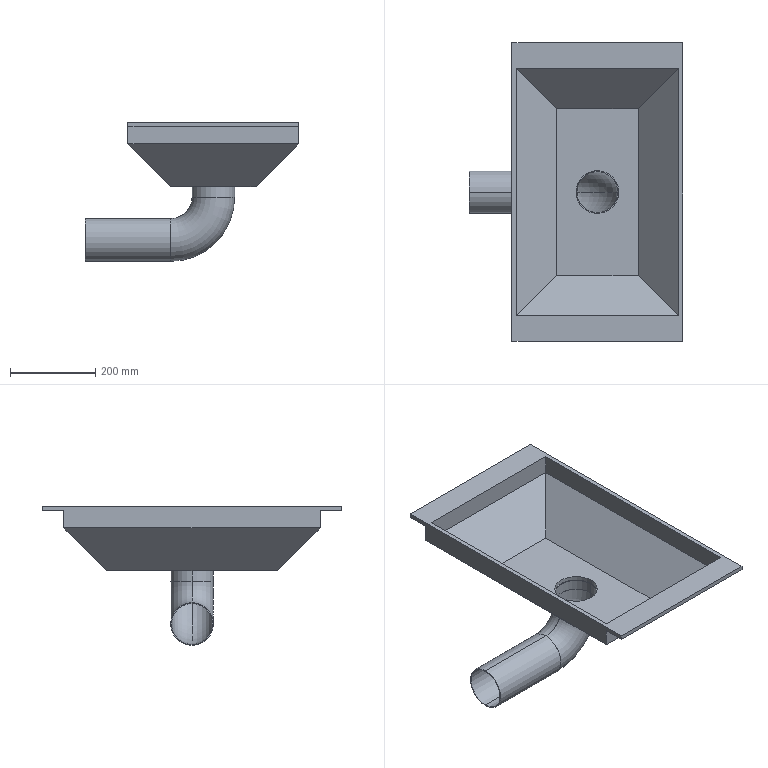Part | SolidWorks | features ICE 4, Shell 2, Chamfer 1, Extrusion 1, Sweep 1 | 2 solids | 39 faces | box 500 x 700 x 325 mm | volume 4429815 mm3 | plane 25 | cylinder 10 | torus 4 | commonest cylinder face diameters 100 x6 96 x4
STEP:
#1=CARTESIAN_POINT('',(48.,0.,-25.));
#2=VERTEX_POINT('',#1);
#3=CARTESIAN_POINT('',(-48.,0.,-25.));
#4=VERTEX_POINT('',#3);
#5=CARTESIAN_POINT('',(0.,0.,-25.));
#6=DIRECTION('',(0.,0.,-1.));
#7=DIRECTION('',(1.,0.,0.));
#8=AXIS2_PLACEMENT_3D('',#5,#6,#7);
#9=CIRCLE('',#8,48.);
#10=EDGE_CURVE('',#2,#4,#9,.T.);
#11=ORIENTED_EDGE('',*,*,#10,.F.);
#12=CARTESIAN_POINT('',(-100.,0.,-173.));
#13=VERTEX_POINT('',#12);
#14=CARTESIAN_POINT('',(-100.,0.,-25.));
#15=DIRECTION('',(0.,1.,0.));
#16=DIRECTION('',(0.,0.,1.));
#17=AXIS2_PLACEMENT_3D('',#14,#15,#16);
#18=CIRCLE('',#17,148.);
#19=EDGE_CURVE('',#2,#13,#18,.T.);
#20=ORIENTED_EDGE('',*,*,#19,.T.);
#21=CARTESIAN_POINT('',(-100.,0.,-77.));
#22=VERTEX_POINT('',#21);
#23=CARTESIAN_POINT('',(-100.,0.,-125.));
#24=DIRECTION('',(-1.,0.,0.));
#25=DIRECTION('',(0.,0.,1.));
#26=AXIS2_PLACEMENT_3D('',#23,#24,#25);
#27=CIRCLE('',#26,48.);
#28=EDGE_CURVE('',#13,#22,#27,.T.);
#29=ORIENTED_EDGE('',*,*,#28,.T.);
#30=CARTESIAN_POINT('',(-100.,0.,-25.));
#31=DIRECTION('',(0.,1.,0.));
#32=DIRECTION('',(0.,0.,1.));
#33=AXIS2_PLACEMENT_3D('',#30,#31,#32);
#34=CIRCLE('',#33,52.);
#35=EDGE_CURVE('',#4,#22,#34,.T.);
#36=ORIENTED_EDGE('',*,*,#35,.F.);
#37=EDGE_LOOP('',(#11,#20,#29,#36));
#38=FACE_OUTER_BOUND('',#37,.T.);
#39=CARTESIAN_POINT('',(-100.,0.,-25.));
#40=DIRECTION('',(0.,1.,0.));
#41=DIRECTION('',(0.,0.,1.));
#42=AXIS2_PLACEMENT_3D('',#39,#40,#41);
#43=TOROIDAL_SURFACE('',#42,100.,48.);
#44=ADVANCED_FACE('',(#38),#43,.F.);
#45=CARTESIAN_POINT('',(-50.,0.,-25.));
#46=VERTEX_POINT('',#45);
#47=CARTESIAN_POINT('',(50.,0.,-25.));
#48=VERTEX_POINT('',#47);
#49=CARTESIAN_POINT('',(0.,0.,-25.));
#50=DIRECTION('',(0.,0.,-1.));
#51=DIRECTION('',(-1.,0.,0.));
#52=AXIS2_PLACEMENT_3D('',#49,#50,#51);
#53=CIRCLE('',#52,50.);
#54=EDGE_CURVE('',#46,#48,#53,.T.);
#55=ORIENTED_EDGE('',*,*,#54,.T.);
#56=CARTESIAN_POINT('',(-100.,0.,-175.));
#57=VERTEX_POINT('',#56);
#58=CARTESIAN_POINT('',(-100.,0.,-25.));
#59=DIRECTION('',(0.,1.,0.));
#60=DIRECTION('',(0.,0.,1.));
#61=AXIS2_PLACEMENT_3D('',#58,#59,#60);
#62=CIRCLE('',#61,150.);
#63=EDGE_CURVE('',#48,#57,#62,.T.);
#64=ORIENTED_EDGE('',*,*,#63,.T.);
#65=CARTESIAN_POINT('',(-100.,0.,-75.));
#66=VERTEX_POINT('',#65);
#67=CARTESIAN_POINT('',(-100.,0.,-125.));
#68=DIRECTION('',(-1.,0.,0.));
#69=DIRECTION('',(0.,0.,1.));
#70=AXIS2_PLACEMENT_3D('',#67,#68,#69);
#71=CIRCLE('',#70,50.);
#72=EDGE_CURVE('',#66,#57,#71,.T.);
#73=ORIENTED_EDGE('',*,*,#72,.F.);
#74=CARTESIAN_POINT('',(-100.,0.,-25.));
#75=DIRECTION('',(0.,1.,0.));
#76=DIRECTION('',(0.,0.,1.));
#77=AXIS2_PLACEMENT_3D('',#74,#75,#76);
#78=CIRCLE('',#77,50.);
#79=EDGE_CURVE('',#46,#66,#78,.T.);
#80=ORIENTED_EDGE('',*,*,#79,.F.);
#81=EDGE_LOOP('',(#55,#64,#73,#80));
#82=FACE_OUTER_BOUND('',#81,.T.);
#83=CARTESIAN_POINT('',(-100.,0.,-25.));
#84=DIRECTION('',(0.,1.,0.));
#85=DIRECTION('',(0.,0.,1.));
#86=AXIS2_PLACEMENT_3D('',#83,#84,#85);
#87=TOROIDAL_SURFACE('',#86,100.,50.);
#88=ADVANCED_FACE('',(#82),#87,.T.);
#89=ORIENTED_EDGE('',*,*,#28,.F.);
#90=CARTESIAN_POINT('',(-300.,0.,-173.));
#91=VERTEX_POINT('',#90);
#92=CARTESIAN_POINT('',(-100.,0.,-173.));
#93=DIRECTION('',(-1.,0.,0.));
#94=VECTOR('',#93,1000.);
#95=LINE('',#92,#94);
#96=EDGE_CURVE('',#13,#91,#95,.T.);
#97=ORIENTED_EDGE('',*,*,#96,.T.);
#98=CARTESIAN_POINT('',(-300.,0.,-77.));
#99=VERTEX_POINT('',#98);
#100=CARTESIAN_POINT('',(-300.,0.,-125.));
#101=DIRECTION('',(-1.,0.,0.));
#102=DIRECTION('',(0.,0.,1.));
#103=AXIS2_PLACEMENT_3D('',#100,#101,#102);
#104=CIRCLE('',#103,48.);
#105=EDGE_CURVE('',#91,#99,#104,.T.);
#106=ORIENTED_EDGE('',*,*,#105,.T.);
#107=CARTESIAN_POINT('',(-100.,0.,-77.));
#108=DIRECTION('',(-1.,0.,0.));
#109=VECTOR('',#108,1000.);
#110=LINE('',#107,#109);
#111=EDGE_CURVE('',#22,#99,#110,.T.);
#112=ORIENTED_EDGE('',*,*,#111,.F.);
#113=EDGE_LOOP('',(#89,#97,#106,#112));
#114=FACE_OUTER_BOUND('',#113,.T.);
#115=CARTESIAN_POINT('',(-100.,0.,-125.));
#116=DIRECTION('',(-1.,0.,0.));
#117=DIRECTION('',(0.,0.,1.));
#118=AXIS2_PLACEMENT_3D('',#115,#116,#117);
#119=CYLINDRICAL_SURFACE('',#118,48.);
#120=ADVANCED_FACE('',(#114),#119,.F.);
#121=CARTESIAN_POINT('',(48.,0.,0.));
#122=VERTEX_POINT('',#121);
#123=CARTESIAN_POINT('',(-48.,0.,0.));
#124=VERTEX_POINT('',#123);
#125=CARTESIAN_POINT('',(0.,0.,0.));
#126=DIRECTION('',(0.,0.,-1.));
#127=DIRECTION('',(-1.,0.,0.));
#128=AXIS2_PLACEMENT_3D('',#125,#126,#127);
#129=CIRCLE('',#128,48.);
#130=EDGE_CURVE('',#122,#124,#129,.T.);
#131=ORIENTED_EDGE('',*,*,#130,.F.);
#132=CARTESIAN_POINT('',(48.,0.,0.));
#133=DIRECTION('',(0.,0.,-1.));
#134=VECTOR('',#133,1000.);
#135=LINE('',#132,#134);
#136=EDGE_CURVE('',#122,#2,#135,.T.);
#137=ORIENTED_EDGE('',*,*,#136,.T.);
#138=ORIENTED_EDGE('',*,*,#10,.T.);
#139=CARTESIAN_POINT('',(-48.,0.,0.));
#140=DIRECTION('',(0.,0.,-1.));
#141=VECTOR('',#140,1000.);
#142=LINE('',#139,#141);
#143=EDGE_CURVE('',#124,#4,#142,.T.);
#144=ORIENTED_EDGE('',*,*,#143,.F.);
#145=EDGE_LOOP('',(#131,#137,#138,#144));
#146=FACE_OUTER_BOUND('',#145,.T.);
#147=CARTESIAN_POINT('',(0.,0.,0.));
#148=DIRECTION('',(0.,0.,-1.));
#149=DIRECTION('',(-1.,0.,0.));
#150=AXIS2_PLACEMENT_3D('',#147,#148,#149);
#151=CYLINDRICAL_SURFACE('',#150,48.);
#152=ADVANCED_FACE('',(#146),#151,.F.);
#153=ORIENTED_EDGE('',*,*,#72,.T.);
#154=CARTESIAN_POINT('',(-300.,0.,-175.));
#155=VERTEX_POINT('',#154);
#156=CARTESIAN_POINT('',(-100.,0.,-175.));
#157=DIRECTION('',(-1.,0.,0.));
#158=VECTOR('',#157,1000.);
#159=LINE('',#156,#158);
#160=EDGE_CURVE('',#57,#155,#159,.T.);
#161=ORIENTED_EDGE('',*,*,#160,.T.);
#162=CARTESIAN_POINT('',(-300.,0.,-75.));
#163=VERTEX_POINT('',#162);
#164=CARTESIAN_POINT('',(-300.,0.,-125.));
#165=DIRECTION('',(-1.,0.,0.));
#166=DIRECTION('',(0.,0.,1.));
#167=AXIS2_PLACEMENT_3D('',#164,#165,#166);
#168=CIRCLE('',#167,50.);
#169=EDGE_CURVE('',#163,#155,#168,.T.);
#170=ORIENTED_EDGE('',*,*,#169,.F.);
#171=CARTESIAN_POINT('',(-100.,0.,-75.));
#172=DIRECTION('',(-1.,0.,0.));
#173=VECTOR('',#172,1000.);
#174=LINE('',#171,#173);
#175=EDGE_CURVE('',#66,#163,#174,.T.);
#176=ORIENTED_EDGE('',*,*,#175,.F.);
#177=EDGE_LOOP('',(#153,#161,#170,#176));
#178=FACE_OUTER_BOUND('',#177,.T.);
#179=CARTESIAN_POINT('',(-100.,0.,-125.));
#180=DIRECTION('',(-1.,0.,0.));
#181=DIRECTION('',(0.,0.,1.));
#182=AXIS2_PLACEMENT_3D('',#179,#180,#181);
#183=CYLINDRICAL_SURFACE('',#182,50.);
#184=ADVANCED_FACE('',(#178),#183,.T.);
#185=CARTESIAN_POINT('',(-50.,0.,0.));
#186=VERTEX_POINT('',#185);
#187=CARTESIAN_POINT('',(50.,0.,0.));
#188=VERTEX_POINT('',#187);
#189=CARTESIAN_POINT('',(0.,0.,0.));
#190=DIRECTION('',(0.,0.,-1.));
#191=DIRECTION('',(-1.,0.,0.));
#192=AXIS2_PLACEMENT_3D('',#189,#190,#191);
#193=CIRCLE('',#192,50.);
#194=EDGE_CURVE('',#186,#188,#193,.T.);
#195=ORIENTED_EDGE('',*,*,#194,.T.);
#196=CARTESIAN_POINT('',(50.,0.,0.));
#197=DIRECTION('',(0.,0.,-1.));
#198=VECTOR('',#197,1000.);
#199=LINE('',#196,#198);
#200=EDGE_CURVE('',#188,#48,#199,.T.);
#201=ORIENTED_EDGE('',*,*,#200,.T.);
#202=ORIENTED_EDGE('',*,*,#54,.F.);
#203=CARTESIAN_POINT('',(-50.,0.,0.));
#204=DIRECTION('',(0.,0.,-1.));
#205=VECTOR('',#204,1000.);
#206=LINE('',#203,#205);
#207=EDGE_CURVE('',#186,#46,#206,.T.);
#208=ORIENTED_EDGE('',*,*,#207,.F.);
#209=EDGE_LOOP('',(#195,#201,#202,#208));
#210=FACE_OUTER_BOUND('',#209,.T.);
#211=CARTESIAN_POINT('',(0.,0.,0.));
#212=DIRECTION('',(0.,0.,-1.));
#213=DIRECTION('',(-1.,0.,0.));
#214=AXIS2_PLACEMENT_3D('',#211,#212,#213);
#215=CYLINDRICAL_SURFACE('',#214,50.);
#216=ADVANCED_FACE('',(#210),#215,.T.);
#217=ORIENTED_EDGE('',*,*,#160,.F.);
#218=CARTESIAN_POINT('',(-100.,0.,-125.));
#219=DIRECTION('',(-1.,0.,0.));
#220=DIRECTION('',(0.,0.,1.));
#221=AXIS2_PLACEMENT_3D('',#218,#219,#220);
#222=CIRCLE('',#221,50.);
#223=EDGE_CURVE('',#57,#66,#222,.T.);
#224=ORIENTED_EDGE('',*,*,#223,.T.);
#225=ORIENTED_EDGE('',*,*,#175,.T.);
#226=CARTESIAN_POINT('',(-300.,0.,-125.));
#227=DIRECTION('',(-1.,0.,0.));
#228=DIRECTION('',(0.,0.,1.));
#229=AXIS2_PLACEMENT_3D('',#226,#227,#228);
#230=CIRCLE('',#229,50.);
#231=EDGE_CURVE('',#155,#163,#230,.T.);
#232=ORIENTED_EDGE('',*,*,#231,.F.);
#233=EDGE_LOOP('',(#217,#224,#225,#232));
#234=FACE_OUTER_BOUND('',#233,.T.);
#235=CARTESIAN_POINT('',(-100.,0.,-125.));
#236=DIRECTION('',(-1.,0.,0.));
#237=DIRECTION('',(0.,0.,1.));
#238=AXIS2_PLACEMENT_3D('',#235,#236,#237);
#239=CYLINDRICAL_SURFACE('',#238,50.);
#240=ADVANCED_FACE('',(#234),#239,.T.);
#241=ORIENTED_EDGE('',*,*,#63,.F.);
#242=CARTESIAN_POINT('',(0.,0.,-25.));
#243=DIRECTION('',(0.,0.,-1.));
#244=DIRECTION('',(-1.,0.,0.));
#245=AXIS2_PLACEMENT_3D('',#242,#243,#244);
#246=CIRCLE('',#245,50.);
#247=EDGE_CURVE('',#48,#46,#246,.T.);
#248=ORIENTED_EDGE('',*,*,#247,.T.);
#249=ORIENTED_EDGE('',*,*,#79,.T.);
#250=ORIENTED_EDGE('',*,*,#223,.F.);
#251=EDGE_LOOP('',(#241,#248,#249,#250));
#252=FACE_OUTER_BOUND('',#251,.T.);
#253=CARTESIAN_POINT('',(-100.,0.,-25.));
#254=DIRECTION('',(0.,1.,0.));
#255=DIRECTION('',(0.,0.,1.));
#256=AXIS2_PLACEMENT_3D('',#253,#254,#255);
#257=TOROIDAL_SURFACE('',#256,100.,50.);
#258=ADVANCED_FACE('',(#252),#257,.T.);
#259=ORIENTED_EDGE('',*,*,#200,.F.);
#260=CARTESIAN_POINT('',(0.,0.,0.));
#261=DIRECTION('',(0.,0.,-1.));
#262=DIRECTION('',(-1.,0.,0.));
#263=AXIS2_PLACEMENT_3D('',#260,#261,#262);
#264=CIRCLE('',#263,50.);
#265=EDGE_CURVE('',#188,#186,#264,.T.);
#266=ORIENTED_EDGE('',*,*,#265,.T.);
#267=ORIENTED_EDGE('',*,*,#207,.T.);
#268=ORIENTED_EDGE('',*,*,#247,.F.);
#269=EDGE_LOOP('',(#259,#266,#267,#268));
#270=FACE_OUTER_BOUND('',#269,.T.);
#271=CARTESIAN_POINT('',(0.,0.,0.));
#272=DIRECTION('',(0.,0.,-1.));
#273=DIRECTION('',(-1.,0.,0.));
#274=AXIS2_PLACEMENT_3D('',#271,#272,#273);
#275=CYLINDRICAL_SURFACE('',#274,50.);
#276=ADVANCED_FACE('',(#270),#275,.T.);
#277=CARTESIAN_POINT('',(-300.,0.,-125.));
#278=DIRECTION('',(-1.,0.,0.));
#279=DIRECTION('',(0.,0.,1.));
#280=AXIS2_PLACEMENT_3D('',#277,#278,#279);
#281=CIRCLE('',#280,48.);
#282=EDGE_CURVE('',#99,#91,#281,.T.);
#283=ORIENTED_EDGE('',*,*,#282,.F.);
#284=ORIENTED_EDGE('',*,*,#105,.F.);
#285=EDGE_LOOP('',(#283,#284));
#286=FACE_BOUND('',#285,.T.);
#287=ORIENTED_EDGE('',*,*,#169,.T.);
#288=ORIENTED_EDGE('',*,*,#231,.T.);
#289=EDGE_LOOP('',(#287,#288));
#290=FACE_OUTER_BOUND('',#289,.T.);
#291=CARTESIAN_POINT('',(-300.,0.,-125.));
#292=DIRECTION('',(-1.,0.,0.));
#293=DIRECTION('',(0.,0.,1.));
#294=AXIS2_PLACEMENT_3D('',#291,#292,#293);
#295=PLANE('',#294);
#296=ADVANCED_FACE('',(#286,#290),#295,.T.);
#297=CARTESIAN_POINT('',(0.,0.,0.));
#298=DIRECTION('',(0.,0.,-1.));
#299=DIRECTION('',(-1.,0.,0.));
#300=AXIS2_PLACEMENT_3D('',#297,#298,#299);
#301=CIRCLE('',#300,48.);
#302=EDGE_CURVE('',#124,#122,#301,.T.);
#303=ORIENTED_EDGE('',*,*,#302,.T.);
#304=ORIENTED_EDGE('',*,*,#130,.T.);
#305=EDGE_LOOP('',(#303,#304));
#306=FACE_BOUND('',#305,.T.);
#307=ORIENTED_EDGE('',*,*,#194,.F.);
#308=ORIENTED_EDGE('',*,*,#265,.F.);
#309=EDGE_LOOP('',(#307,#308));
#310=FACE_OUTER_BOUND('',#309,.T.);
#311=CARTESIAN_POINT('',(0.,0.,0.));
#312=DIRECTION('',(0.,0.,-1.));
#313=DIRECTION('',(-1.,0.,0.));
#314=AXIS2_PLACEMENT_3D('',#311,#312,#313);
#315=PLANE('',#314);
#316=ADVANCED_FACE('',(#306,#310),#315,.F.);
#317=ORIENTED_EDGE('',*,*,#96,.F.);
#318=CARTESIAN_POINT('',(-100.,0.,-125.));
#319=DIRECTION('',(-1.,0.,0.));
#320=DIRECTION('',(0.,0.,1.));
#321=AXIS2_PLACEMENT_3D('',#318,#319,#320);
#322=CIRCLE('',#321,48.);
#323=EDGE_CURVE('',#22,#13,#322,.T.);
#324=ORIENTED_EDGE('',*,*,#323,.F.);
#325=ORIENTED_EDGE('',*,*,#111,.T.);
#326=ORIENTED_EDGE('',*,*,#282,.T.);
#327=EDGE_LOOP('',(#317,#324,#325,#326));
#328=FACE_OUTER_BOUND('',#327,.T.);
#329=CARTESIAN_POINT('',(-100.,0.,-125.));
#330=DIRECTION('',(-1.,0.,0.));
#331=DIRECTION('',(0.,0.,1.));
#332=AXIS2_PLACEMENT_3D('',#329,#330,#331);
#333=CYLINDRICAL_SURFACE('',#332,48.);
#334=ADVANCED_FACE('',(#328),#333,.F.);
#335=ORIENTED_EDGE('',*,*,#19,.F.);
#336=CARTESIAN_POINT('',(0.,0.,-25.));
#337=DIRECTION('',(0.,0.,-1.));
#338=DIRECTION('',(1.,0.,0.));
#339=AXIS2_PLACEMENT_3D('',#336,#337,#338);
#340=CIRCLE('',#339,48.);
#341=EDGE_CURVE('',#4,#2,#340,.T.);
#342=ORIENTED_EDGE('',*,*,#341,.F.);
#343=ORIENTED_EDGE('',*,*,#35,.T.);
#344=ORIENTED_EDGE('',*,*,#323,.T.);
#345=EDGE_LOOP('',(#335,#342,#343,#344));
#346=FACE_OUTER_BOUND('',#345,.T.);
#347=CARTESIAN_POINT('',(-100.,0.,-25.));
#348=DIRECTION('',(0.,1.,0.));
#349=DIRECTION('',(0.,0.,1.));
#350=AXIS2_PLACEMENT_3D('',#347,#348,#349);
#351=TOROIDAL_SURFACE('',#350,100.,48.);
#352=ADVANCED_FACE('',(#346),#351,.F.);
#353=ORIENTED_EDGE('',*,*,#136,.F.);
#354=ORIENTED_EDGE('',*,*,#302,.F.);
#355=ORIENTED_EDGE('',*,*,#143,.T.);
#356=ORIENTED_EDGE('',*,*,#341,.T.);
#357=EDGE_LOOP('',(#353,#354,#355,#356));
#358=FACE_OUTER_BOUND('',#357,.T.);
#359=CARTESIAN_POINT('',(0.,0.,0.));
#360=DIRECTION('',(0.,0.,-1.));
#361=DIRECTION('',(-1.,0.,0.));
#362=AXIS2_PLACEMENT_3D('',#359,#360,#361);
#363=CYLINDRICAL_SURFACE('',#362,48.);
#364=ADVANCED_FACE('',(#358),#363,.F.);
#365=CLOSED_SHELL('',(#44,#88,#120,#152,#184,#216,#240,#258,#276,#296,#316,#334,#352,#364));
#366=MANIFOLD_SOLID_BREP('',#365);
#367=CARTESIAN_POINT('',(-50.,0.,0.));
#368=VERTEX_POINT('',#367);
#369=CARTESIAN_POINT('',(50.,0.,0.));
#370=VERTEX_POINT('',#369);
#371=CARTESIAN_POINT('',(0.,0.,0.));
#372=DIRECTION('',(0.,0.,1.));
#373=DIRECTION('',(1.,0.,0.));
#374=AXIS2_PLACEMENT_3D('',#371,#372,#373);
#375=CIRCLE('',#374,50.);
#376=EDGE_CURVE('',#368,#370,#375,.T.);
#377=ORIENTED_EDGE('',*,*,#376,.F.);
#378=CARTESIAN_POINT('',(-50.,0.,10.));
#379=VERTEX_POINT('',#378);
#380=CARTESIAN_POINT('',(-50.,0.,0.));
#381=DIRECTION('',(0.,0.,1.));
#382=VECTOR('',#381,1000.);
#383=LINE('',#380,#382);
#384=EDGE_CURVE('',#368,#379,#383,.T.);
#385=ORIENTED_EDGE('',*,*,#384,.T.);
#386=CARTESIAN_POINT('',(50.,0.,10.));
#387=VERTEX_POINT('',#386);
#388=CARTESIAN_POINT('',(0.,0.,10.));
#389=DIRECTION('',(0.,0.,1.));
#390=DIRECTION('',(1.,0.,0.));
#391=AXIS2_PLACEMENT_3D('',#388,#389,#390);
#392=CIRCLE('',#391,50.);
#393=EDGE_CURVE('',#379,#387,#392,.T.);
#394=ORIENTED_EDGE('',*,*,#393,.T.);
#395=CARTESIAN_POINT('',(50.,0.,0.));
#396=DIRECTION('',(0.,0.,1.));
#397=VECTOR('',#396,1000.);
#398=LINE('',#395,#397);
#399=EDGE_CURVE('',#370,#387,#398,.T.);
#400=ORIENTED_EDGE('',*,*,#399,.F.);
#401=EDGE_LOOP('',(#377,#385,#394,#400));
#402=FACE_OUTER_BOUND('',#401,.T.);
#403=CARTESIAN_POINT('',(0.,0.,0.));
#404=DIRECTION('',(0.,0.,1.));
#405=DIRECTION('',(1.,0.,0.));
#406=AXIS2_PLACEMENT_3D('',#403,#404,#405);
#407=CYLINDRICAL_SURFACE('',#406,50.);
#408=ADVANCED_FACE('',(#402),#407,.F.);
#409=CARTESIAN_POINT('',(200.,-350.,150.));
#410=VERTEX_POINT('',#409);
#411=CARTESIAN_POINT('',(200.,350.,150.));
#412=VERTEX_POINT('',#411);
#413=CARTESIAN_POINT('',(200.,-300.,150.));
#414=DIRECTION('',(0.,1.,0.));
#415=VECTOR('',#414,1000.);
#416=LINE('',#413,#415);
#417=EDGE_CURVE('',#410,#412,#416,.T.);
#418=ORIENTED_EDGE('',*,*,#417,.T.);
#419=CARTESIAN_POINT('',(-200.,350.,150.));
#420=VERTEX_POINT('',#419);
#421=CARTESIAN_POINT('',(-200.,350.,150.));
#422=DIRECTION('',(-1.,0.,0.));
#423=VECTOR('',#422,1000.);
#424=LINE('',#421,#423);
#425=EDGE_CURVE('',#412,#420,#424,.T.);
#426=ORIENTED_EDGE('',*,*,#425,.T.);
#427=CARTESIAN_POINT('',(-200.,-350.,150.));
#428=VERTEX_POINT('',#427);
#429=CARTESIAN_POINT('',(-200.,-300.,150.));
#430=DIRECTION('',(0.,-1.,0.));
#431=VECTOR('',#430,1000.);
#432=LINE('',#429,#431);
#433=EDGE_CURVE('',#420,#428,#432,.T.);
#434=ORIENTED_EDGE('',*,*,#433,.T.);
#435=CARTESIAN_POINT('',(-200.,-350.,150.));
#436=DIRECTION('',(1.,0.,0.));
#437=VECTOR('',#436,1000.);
#438=LINE('',#435,#437);
#439=EDGE_CURVE('',#428,#410,#438,.T.);
#440=ORIENTED_EDGE('',*,*,#439,.T.);
#441=EDGE_LOOP('',(#418,#426,#434,#440));
#442=FACE_OUTER_BOUND('',#441,.T.);
#443=CARTESIAN_POINT('',(190.,-290.,150.));
#444=VERTEX_POINT('',#443);
#445=CARTESIAN_POINT('',(190.,290.,150.));
#446=VERTEX_POINT('',#445);
#447=CARTESIAN_POINT('',(190.,0.,150.));
#448=DIRECTION('',(0.,1.,0.));
#449=VECTOR('',#448,1000.);
#450=LINE('',#447,#449);
#451=EDGE_CURVE('',#444,#446,#450,.T.);
#452=ORIENTED_EDGE('',*,*,#451,.F.);
#453=CARTESIAN_POINT('',(-190.,-290.,150.));
#454=VERTEX_POINT('',#453);
#455=CARTESIAN_POINT('',(0.,-290.,150.));
#456=DIRECTION('',(1.,0.,0.));
#457=VECTOR('',#456,1000.);
#458=LINE('',#455,#457);
#459=EDGE_CURVE('',#454,#444,#458,.T.);
#460=ORIENTED_EDGE('',*,*,#459,.F.);
#461=CARTESIAN_POINT('',(-190.,290.,150.));
#462=VERTEX_POINT('',#461);
#463=CARTESIAN_POINT('',(-190.,0.,150.));
#464=DIRECTION('',(0.,-1.,0.));
#465=VECTOR('',#464,1000.);
#466=LINE('',#463,#465);
#467=EDGE_CURVE('',#462,#454,#466,.T.);
#468=ORIENTED_EDGE('',*,*,#467,.F.);
#469=CARTESIAN_POINT('',(0.,290.,150.));
#470=DIRECTION('',(-1.,0.,0.));
#471=VECTOR('',#470,1000.);
#472=LINE('',#469,#471);
#473=EDGE_CURVE('',#446,#462,#472,.T.);
#474=ORIENTED_EDGE('',*,*,#473,.F.);
#475=EDGE_LOOP('',(#452,#460,#468,#474));
#476=FACE_BOUND('',#475,.T.);
#477=CARTESIAN_POINT('',(0.,0.,150.));
#478=DIRECTION('',(0.,0.,-1.));
#479=DIRECTION('',(-1.,0.,0.));
#480=AXIS2_PLACEMENT_3D('',#477,#478,#479);
#481=PLANE('',#480);
#482=ADVANCED_FACE('',(#442,#476),#481,.F.);
#483=ORIENTED_EDGE('',*,*,#417,.F.);
#484=CARTESIAN_POINT('',(200.,-350.,140.));
#485=VERTEX_POINT('',#484);
#486=CARTESIAN_POINT('',(200.,-350.,140.));
#487=DIRECTION('',(0.,0.,1.));
#488=VECTOR('',#487,1000.);
#489=LINE('',#486,#488);
#490=EDGE_CURVE('',#485,#410,#489,.T.);
#491=ORIENTED_EDGE('',*,*,#490,.F.);
#492=CARTESIAN_POINT('',(200.,-300.,140.));
#493=VERTEX_POINT('',#492);
#494=CARTESIAN_POINT('',(200.,-300.,140.));
#495=DIRECTION('',(0.,1.,0.));
#496=VECTOR('',#495,1000.);
#497=LINE('',#494,#496);
#498=EDGE_CURVE('',#485,#493,#497,.T.);
#499=ORIENTED_EDGE('',*,*,#498,.T.);
#500=CARTESIAN_POINT('',(200.,-300.,100.));
#501=VERTEX_POINT('',#500);
#502=CARTESIAN_POINT('',(200.,-300.,150.));
#503=DIRECTION('',(0.,0.,-1.));
#504=VECTOR('',#503,1000.);
#505=LINE('',#502,#504);
#506=EDGE_CURVE('',#493,#501,#505,.T.);
#507=ORIENTED_EDGE('',*,*,#506,.T.);
#508=CARTESIAN_POINT('',(200.,300.,100.));
#509=VERTEX_POINT('',#508);
#510=CARTESIAN_POINT('',(200.,300.,100.));
#511=DIRECTION('',(0.,1.,0.));
#512=VECTOR('',#511,1000.);
#513=LINE('',#510,#512);
#514=EDGE_CURVE('',#501,#509,#513,.T.);
#515=ORIENTED_EDGE('',*,*,#514,.T.);
#516=CARTESIAN_POINT('',(200.,300.,140.));
#517=VERTEX_POINT('',#516);
#518=CARTESIAN_POINT('',(200.,300.,150.));
#519=DIRECTION('',(0.,0.,-1.));
#520=VECTOR('',#519,1000.);
#521=LINE('',#518,#520);
#522=EDGE_CURVE('',#517,#509,#521,.T.);
#523=ORIENTED_EDGE('',*,*,#522,.F.);
#524=CARTESIAN_POINT('',(200.,350.,140.));
#525=VERTEX_POINT('',#524);
#526=CARTESIAN_POINT('',(200.,300.,140.));
#527=DIRECTION('',(0.,1.,0.));
#528=VECTOR('',#527,1000.);
#529=LINE('',#526,#528);
#530=EDGE_CURVE('',#517,#525,#529,.T.);
#531=ORIENTED_EDGE('',*,*,#530,.T.);
#532=CARTESIAN_POINT('',(200.,350.,140.));
#533=DIRECTION('',(0.,0.,1.));
#534=VECTOR('',#533,1000.);
#535=LINE('',#532,#534);
#536=EDGE_CURVE('',#525,#412,#535,.T.);
#537=ORIENTED_EDGE('',*,*,#536,.T.);
#538=EDGE_LOOP('',(#483,#491,#499,#507,#515,#523,#531,#537));
#539=FACE_OUTER_BOUND('',#538,.T.);
#540=CARTESIAN_POINT('',(200.,-300.,150.));
#541=DIRECTION('',(-1.,0.,0.));
#542=DIRECTION('',(0.,0.,1.));
#543=AXIS2_PLACEMENT_3D('',#540,#541,#542);
#544=PLANE('',#543);
#545=ADVANCED_FACE('',(#539),#544,.F.);
#546=CARTESIAN_POINT('',(-200.,300.,140.));
#547=VERTEX_POINT('',#546);
#548=CARTESIAN_POINT('',(-200.,300.,100.));
#549=VERTEX_POINT('',#548);
#550=CARTESIAN_POINT('',(-200.,300.,150.));
#551=DIRECTION('',(0.,0.,-1.));
#552=VECTOR('',#551,1000.);
#553=LINE('',#550,#552);
#554=EDGE_CURVE('',#547,#549,#553,.T.);
#555=ORIENTED_EDGE('',*,*,#554,.F.);
#556=CARTESIAN_POINT('',(-200.,300.,140.));
#557=DIRECTION('',(1.,0.,0.));
#558=VECTOR('',#557,1000.);
#559=LINE('',#556,#558);
#560=EDGE_CURVE('',#547,#517,#559,.T.);
#561=ORIENTED_EDGE('',*,*,#560,.T.);
#562=ORIENTED_EDGE('',*,*,#522,.T.);
#563=CARTESIAN_POINT('',(-200.,300.,100.));
#564=DIRECTION('',(-1.,0.,0.));
#565=VECTOR('',#564,1000.);
#566=LINE('',#563,#565);
#567=EDGE_CURVE('',#509,#549,#566,.T.);
#568=ORIENTED_EDGE('',*,*,#567,.T.);
#569=EDGE_LOOP('',(#555,#561,#562,#568));
#570=FACE_OUTER_BOUND('',#569,.T.);
#571=CARTESIAN_POINT('',(-200.,300.,150.));
#572=DIRECTION('',(0.,-1.,0.));
#573=DIRECTION('',(0.,0.,-1.));
#574=AXIS2_PLACEMENT_3D('',#571,#572,#573);
#575=PLANE('',#574);
#576=ADVANCED_FACE('',(#570),#575,.F.);
#577=ORIENTED_EDGE('',*,*,#433,.F.);
#578=CARTESIAN_POINT('',(-200.,350.,140.));
#579=VERTEX_POINT('',#578);
#580=CARTESIAN_POINT('',(-200.,350.,140.));
#581=DIRECTION('',(0.,0.,1.));
#582=VECTOR('',#581,1000.);
#583=LINE('',#580,#582);
#584=EDGE_CURVE('',#579,#420,#583,.T.);
#585=ORIENTED_EDGE('',*,*,#584,.F.);
#586=CARTESIAN_POINT('',(-200.,300.,140.));
#587=DIRECTION('',(0.,-1.,0.));
#588=VECTOR('',#587,1000.);
#589=LINE('',#586,#588);
#590=EDGE_CURVE('',#579,#547,#589,.T.);
#591=ORIENTED_EDGE('',*,*,#590,.T.);
#592=ORIENTED_EDGE('',*,*,#554,.T.);
#593=CARTESIAN_POINT('',(-200.,-300.,100.));
#594=VERTEX_POINT('',#593);
#595=CARTESIAN_POINT('',(-200.,-300.,100.));
#596=DIRECTION('',(0.,-1.,0.));
#597=VECTOR('',#596,1000.);
#598=LINE('',#595,#597);
#599=EDGE_CURVE('',#549,#594,#598,.T.);
#600=ORIENTED_EDGE('',*,*,#599,.T.);
#601=CARTESIAN_POINT('',(-200.,-300.,140.));
#602=VERTEX_POINT('',#601);
#603=CARTESIAN_POINT('',(-200.,-300.,150.));
#604=DIRECTION('',(0.,0.,-1.));
#605=VECTOR('',#604,1000.);
#606=LINE('',#603,#605);
#607=EDGE_CURVE('',#602,#594,#606,.T.);
#608=ORIENTED_EDGE('',*,*,#607,.F.);
#609=CARTESIAN_POINT('',(-200.,-350.,140.));
#610=VERTEX_POINT('',#609);
#611=CARTESIAN_POINT('',(-200.,-300.,140.));
#612=DIRECTION('',(0.,-1.,0.));
#613=VECTOR('',#612,1000.);
#614=LINE('',#611,#613);
#615=EDGE_CURVE('',#602,#610,#614,.T.);
#616=ORIENTED_EDGE('',*,*,#615,.T.);
#617=CARTESIAN_POINT('',(-200.,-350.,140.));
#618=DIRECTION('',(0.,0.,1.));
#619=VECTOR('',#618,1000.);
#620=LINE('',#617,#619);
#621=EDGE_CURVE('',#610,#428,#620,.T.);
#622=ORIENTED_EDGE('',*,*,#621,.T.);
#623=EDGE_LOOP('',(#577,#585,#591,#592,#600,#608,#616,#622));
#624=FACE_OUTER_BOUND('',#623,.T.);
#625=CARTESIAN_POINT('',(-200.,-300.,150.));
#626=DIRECTION('',(1.,0.,0.));
#627=DIRECTION('',(0.,0.,-1.));
#628=AXIS2_PLACEMENT_3D('',#625,#626,#627);
#629=PLANE('',#628);
#630=ADVANCED_FACE('',(#624),#629,.F.);
#631=ORIENTED_EDGE('',*,*,#506,.F.);
#632=CARTESIAN_POINT('',(-200.,-300.,140.));
#633=DIRECTION('',(-1.,0.,0.));
#634=VECTOR('',#633,1000.);
#635=LINE('',#632,#634);
#636=EDGE_CURVE('',#493,#602,#635,.T.);
#637=ORIENTED_EDGE('',*,*,#636,.T.);
#638=ORIENTED_EDGE('',*,*,#607,.T.);
#639=CARTESIAN_POINT('',(200.,-300.,100.));
#640=DIRECTION('',(1.,0.,0.));
#641=VECTOR('',#640,1000.);
#642=LINE('',#639,#641);
#643=EDGE_CURVE('',#594,#501,#642,.T.);
#644=ORIENTED_EDGE('',*,*,#643,.T.);
#645=EDGE_LOOP('',(#631,#637,#638,#644));
#646=FACE_OUTER_BOUND('',#645,.T.);
#647=CARTESIAN_POINT('',(-200.,-300.,150.));
#648=DIRECTION('',(0.,1.,0.));
#649=DIRECTION('',(0.,0.,1.));
#650=AXIS2_PLACEMENT_3D('',#647,#648,#649);
#651=PLANE('',#650);
#652=ADVANCED_FACE('',(#646),#651,.F.);
#653=CARTESIAN_POINT('',(0.,0.,0.));
#654=DIRECTION('',(0.,0.,1.));
#655=DIRECTION('',(1.,0.,0.));
#656=AXIS2_PLACEMENT_3D('',#653,#654,#655);
#657=CIRCLE('',#656,50.);
#658=EDGE_CURVE('',#370,#368,#657,.T.);
#659=ORIENTED_EDGE('',*,*,#658,.T.);
#660=ORIENTED_EDGE('',*,*,#376,.T.);
#661=EDGE_LOOP('',(#659,#660));
#662=FACE_BOUND('',#661,.T.);
#663=CARTESIAN_POINT('',(-100.,-200.,0.));
#664=VERTEX_POINT('',#663);
#665=CARTESIAN_POINT('',(-100.,200.,0.));
#666=VERTEX_POINT('',#665);
#667=CARTESIAN_POINT('',(-100.,300.,0.));
#668=DIRECTION('',(0.,1.,0.));
#669=VECTOR('',#668,1000.);
#670=LINE('',#667,#669);
#671=EDGE_CURVE('',#664,#666,#670,.T.);
#672=ORIENTED_EDGE('',*,*,#671,.T.);
#673=CARTESIAN_POINT('',(100.,200.,0.));
#674=VERTEX_POINT('',#673);
#675=CARTESIAN_POINT('',(200.,200.,0.));
#676=DIRECTION('',(1.,0.,0.));
#677=VECTOR('',#676,1000.);
#678=LINE('',#675,#677);
#679=EDGE_CURVE('',#666,#674,#678,.T.);
#680=ORIENTED_EDGE('',*,*,#679,.T.);
#681=CARTESIAN_POINT('',(100.,-200.,0.));
#682=VERTEX_POINT('',#681);
#683=CARTESIAN_POINT('',(100.,-300.,0.));
#684=DIRECTION('',(0.,-1.,0.));
#685=VECTOR('',#684,1000.);
#686=LINE('',#683,#685);
#687=EDGE_CURVE('',#674,#682,#686,.T.);
#688=ORIENTED_EDGE('',*,*,#687,.T.);
#689=CARTESIAN_POINT('',(-200.,-200.,0.));
#690=DIRECTION('',(-1.,0.,0.));
#691=VECTOR('',#690,1000.);
#692=LINE('',#689,#691);
#693=EDGE_CURVE('',#682,#664,#692,.T.);
#694=ORIENTED_EDGE('',*,*,#693,.T.);
#695=EDGE_LOOP('',(#672,#680,#688,#694));
#696=FACE_OUTER_BOUND('',#695,.T.);
#697=CARTESIAN_POINT('',(0.,0.,0.));
#698=DIRECTION('',(0.,0.,-1.));
#699=DIRECTION('',(-1.,0.,0.));
#700=AXIS2_PLACEMENT_3D('',#697,#698,#699);
#701=PLANE('',#700);
#702=ADVANCED_FACE('',(#662,#696),#701,.T.);
#703=CARTESIAN_POINT('',(-200.,-300.,100.));
#704=DIRECTION('',(-0.5774,-0.5774,0.5774));
#705=VECTOR('',#704,1000.);
#706=LINE('',#703,#705);
#707=EDGE_CURVE('',#664,#594,#706,.T.);
#708=ORIENTED_EDGE('',*,*,#707,.F.);
#709=ORIENTED_EDGE('',*,*,#693,.F.);
#710=CARTESIAN_POINT('',(200.,-300.,100.));
#711=DIRECTION('',(-0.5774,0.5774,-0.5774));
#712=VECTOR('',#711,1000.);
#713=LINE('',#710,#712);
#714=EDGE_CURVE('',#501,#682,#713,.T.);
#715=ORIENTED_EDGE('',*,*,#714,.F.);
#716=ORIENTED_EDGE('',*,*,#643,.F.);
#717=EDGE_LOOP('',(#708,#709,#715,#716));
#718=FACE_OUTER_BOUND('',#717,.T.);
#719=CARTESIAN_POINT('',(-200.,-300.,100.));
#720=DIRECTION('',(0.,-0.7071,-0.7071));
#721=DIRECTION('',(-1.,0.,0.));
#722=AXIS2_PLACEMENT_3D('',#719,#720,#721);
#723=PLANE('',#722);
#724=ADVANCED_FACE('',(#718),#723,.T.);
#725=ORIENTED_EDGE('',*,*,#714,.T.);
#726=ORIENTED_EDGE('',*,*,#687,.F.);
#727=CARTESIAN_POINT('',(0.,100.,-100.));
#728=DIRECTION('',(-0.5774,-0.5774,-0.5774));
#729=VECTOR('',#728,1000.);
#730=LINE('',#727,#729);
#731=EDGE_CURVE('',#509,#674,#730,.T.);
#732=ORIENTED_EDGE('',*,*,#731,.F.);
#733=ORIENTED_EDGE('',*,*,#514,.F.);
#734=EDGE_LOOP('',(#725,#726,#732,#733));
#735=FACE_OUTER_BOUND('',#734,.T.);
#736=CARTESIAN_POINT('',(200.,-300.,100.));
#737=DIRECTION('',(0.7071,0.,-0.7071));
#738=DIRECTION('',(0.,-1.,0.));
#739=AXIS2_PLACEMENT_3D('',#736,#737,#738);
#740=PLANE('',#739);
#741=ADVANCED_FACE('',(#735),#740,.T.);
#742=ORIENTED_EDGE('',*,*,#707,.T.);
#743=ORIENTED_EDGE('',*,*,#599,.F.);
#744=CARTESIAN_POINT('',(0.,100.,-100.));
#745=DIRECTION('',(-0.5774,0.5774,0.5774));
#746=VECTOR('',#745,1000.);
#747=LINE('',#744,#746);
#748=EDGE_CURVE('',#666,#549,#747,.T.);
#749=ORIENTED_EDGE('',*,*,#748,.F.);
#750=ORIENTED_EDGE('',*,*,#671,.F.);
#751=EDGE_LOOP('',(#742,#743,#749,#750));
#752=FACE_OUTER_BOUND('',#751,.T.);
#753=CARTESIAN_POINT('',(-200.,-300.,100.));
#754=DIRECTION('',(-0.7071,0.,-0.7071));
#755=DIRECTION('',(0.,1.,0.));
#756=AXIS2_PLACEMENT_3D('',#753,#754,#755);
#757=PLANE('',#756);
#758=ADVANCED_FACE('',(#752),#757,.T.);
#759=ORIENTED_EDGE('',*,*,#731,.T.);
#760=ORIENTED_EDGE('',*,*,#679,.F.);
#761=ORIENTED_EDGE('',*,*,#748,.T.);
#762=ORIENTED_EDGE('',*,*,#567,.F.);
#763=EDGE_LOOP('',(#759,#760,#761,#762));
#764=FACE_OUTER_BOUND('',#763,.T.);
#765=CARTESIAN_POINT('',(-200.,300.,100.));
#766=DIRECTION('',(0.,0.7071,-0.7071));
#767=DIRECTION('',(1.,0.,0.));
#768=AXIS2_PLACEMENT_3D('',#765,#766,#767);
#769=PLANE('',#768);
#770=ADVANCED_FACE('',(#764),#769,.T.);
#771=CARTESIAN_POINT('',(190.,-290.,104.142));
#772=VERTEX_POINT('',#771);
#773=CARTESIAN_POINT('',(190.,-290.,150.));
#774=DIRECTION('',(0.,0.,-1.));
#775=VECTOR('',#774,1000.);
#776=LINE('',#773,#775);
#777=EDGE_CURVE('',#444,#772,#776,.T.);
#778=ORIENTED_EDGE('',*,*,#777,.F.);
#779=ORIENTED_EDGE('',*,*,#451,.T.);
#780=CARTESIAN_POINT('',(190.,290.,104.142));
#781=VERTEX_POINT('',#780);
#782=CARTESIAN_POINT('',(190.,290.,150.));
#783=DIRECTION('',(0.,0.,-1.));
#784=VECTOR('',#783,1000.);
#785=LINE('',#782,#784);
#786=EDGE_CURVE('',#446,#781,#785,.T.);
#787=ORIENTED_EDGE('',*,*,#786,.T.);
#788=CARTESIAN_POINT('',(190.,-300.,104.142));
#789=DIRECTION('',(0.,1.,0.));
#790=VECTOR('',#789,1000.);
#791=LINE('',#788,#790);
#792=EDGE_CURVE('',#772,#781,#791,.T.);
#793=ORIENTED_EDGE('',*,*,#792,.F.);
#794=EDGE_LOOP('',(#778,#779,#787,#793));
#795=FACE_OUTER_BOUND('',#794,.T.);
#796=CARTESIAN_POINT('',(190.,-300.,150.));
#797=DIRECTION('',(-1.,0.,0.));
#798=DIRECTION('',(0.,0.,1.));
#799=AXIS2_PLACEMENT_3D('',#796,#797,#798);
#800=PLANE('',#799);
#801=ADVANCED_FACE('',(#795),#800,.T.);
#802=ORIENTED_EDGE('',*,*,#786,.F.);
#803=ORIENTED_EDGE('',*,*,#473,.T.);
#804=CARTESIAN_POINT('',(-190.,290.,104.142));
#805=VERTEX_POINT('',#804);
#806=CARTESIAN_POINT('',(-190.,290.,150.));
#807=DIRECTION('',(0.,0.,-1.));
#808=VECTOR('',#807,1000.);
#809=LINE('',#806,#808);
#810=EDGE_CURVE('',#462,#805,#809,.T.);
#811=ORIENTED_EDGE('',*,*,#810,.T.);
#812=CARTESIAN_POINT('',(-200.,290.,104.142));
#813=DIRECTION('',(-1.,0.,0.));
#814=VECTOR('',#813,1000.);
#815=LINE('',#812,#814);
#816=EDGE_CURVE('',#781,#805,#815,.T.);
#817=ORIENTED_EDGE('',*,*,#816,.F.);
#818=EDGE_LOOP('',(#802,#803,#811,#817));
#819=FACE_OUTER_BOUND('',#818,.T.);
#820=CARTESIAN_POINT('',(-200.,290.,150.));
#821=DIRECTION('',(0.,-1.,0.));
#822=DIRECTION('',(0.,0.,-1.));
#823=AXIS2_PLACEMENT_3D('',#820,#821,#822);
#824=PLANE('',#823);
#825=ADVANCED_FACE('',(#819),#824,.T.);
#826=ORIENTED_EDGE('',*,*,#810,.F.);
#827=ORIENTED_EDGE('',*,*,#467,.T.);
#828=CARTESIAN_POINT('',(-190.,-290.,104.142));
#829=VERTEX_POINT('',#828);
#830=CARTESIAN_POINT('',(-190.,-290.,150.));
#831=DIRECTION('',(0.,0.,-1.));
#832=VECTOR('',#831,1000.);
#833=LINE('',#830,#832);
#834=EDGE_CURVE('',#454,#829,#833,.T.);
#835=ORIENTED_EDGE('',*,*,#834,.T.);
#836=CARTESIAN_POINT('',(-190.,-300.,104.142));
#837=DIRECTION('',(0.,-1.,0.));
#838=VECTOR('',#837,1000.);
#839=LINE('',#836,#838);
#840=EDGE_CURVE('',#805,#829,#839,.T.);
#841=ORIENTED_EDGE('',*,*,#840,.F.);
#842=EDGE_LOOP('',(#826,#827,#835,#841));
#843=FACE_OUTER_BOUND('',#842,.T.);
#844=CARTESIAN_POINT('',(-190.,-300.,150.));
#845=DIRECTION('',(1.,0.,0.));
#846=DIRECTION('',(0.,0.,-1.));
#847=AXIS2_PLACEMENT_3D('',#844,#845,#846);
#848=PLANE('',#847);
#849=ADVANCED_FACE('',(#843),#848,.T.);
#850=ORIENTED_EDGE('',*,*,#834,.F.);
#851=ORIENTED_EDGE('',*,*,#459,.T.);
#852=ORIENTED_EDGE('',*,*,#777,.T.);
#853=CARTESIAN_POINT('',(-200.,-290.,104.142));
#854=DIRECTION('',(1.,0.,0.));
#855=VECTOR('',#854,1000.);
#856=LINE('',#853,#855);
#857=EDGE_CURVE('',#829,#772,#856,.T.);
#858=ORIENTED_EDGE('',*,*,#857,.F.);
#859=EDGE_LOOP('',(#850,#851,#852,#858));
#860=FACE_OUTER_BOUND('',#859,.T.);
#861=CARTESIAN_POINT('',(-200.,-290.,150.));
#862=DIRECTION('',(0.,1.,0.));
#863=DIRECTION('',(0.,0.,1.));
#864=AXIS2_PLACEMENT_3D('',#861,#862,#863);
#865=PLANE('',#864);
#866=ADVANCED_FACE('',(#860),#865,.T.);
#867=CARTESIAN_POINT('',(0.,0.,10.));
#868=DIRECTION('',(0.,0.,1.));
#869=DIRECTION('',(1.,0.,0.));
#870=AXIS2_PLACEMENT_3D('',#867,#868,#869);
#871=CIRCLE('',#870,50.);
#872=EDGE_CURVE('',#387,#379,#871,.T.);
#873=ORIENTED_EDGE('',*,*,#872,.F.);
#874=ORIENTED_EDGE('',*,*,#393,.F.);
#875=EDGE_LOOP('',(#873,#874));
#876=FACE_BOUND('',#875,.T.);
#877=CARTESIAN_POINT('',(-95.858,-195.858,10.));
#878=VERTEX_POINT('',#877);
#879=CARTESIAN_POINT('',(-95.858,195.858,10.));
#880=VERTEX_POINT('',#879);
#881=CARTESIAN_POINT('',(-95.858,0.,10.));
#882=DIRECTION('',(0.,1.,0.));
#883=VECTOR('',#882,1000.);
#884=LINE('',#881,#883);
#885=EDGE_CURVE('',#878,#880,#884,.T.);
#886=ORIENTED_EDGE('',*,*,#885,.F.);
#887=CARTESIAN_POINT('',(95.858,-195.858,10.));
#888=VERTEX_POINT('',#887);
#889=CARTESIAN_POINT('',(0.,-195.858,10.));
#890=DIRECTION('',(-1.,0.,0.));
#891=VECTOR('',#890,1000.);
#892=LINE('',#889,#891);
#893=EDGE_CURVE('',#888,#878,#892,.T.);
#894=ORIENTED_EDGE('',*,*,#893,.F.);
#895=CARTESIAN_POINT('',(95.858,195.858,10.));
#896=VERTEX_POINT('',#895);
#897=CARTESIAN_POINT('',(95.858,0.,10.));
#898=DIRECTION('',(0.,-1.,0.));
#899=VECTOR('',#898,1000.);
#900=LINE('',#897,#899);
#901=EDGE_CURVE('',#896,#888,#900,.T.);
#902=ORIENTED_EDGE('',*,*,#901,.F.);
#903=CARTESIAN_POINT('',(0.,195.858,10.));
#904=DIRECTION('',(1.,0.,0.));
#905=VECTOR('',#904,1000.);
#906=LINE('',#903,#905);
#907=EDGE_CURVE('',#880,#896,#906,.T.);
#908=ORIENTED_EDGE('',*,*,#907,.F.);
#909=EDGE_LOOP('',(#886,#894,#902,#908));
#910=FACE_OUTER_BOUND('',#909,.T.);
#911=CARTESIAN_POINT('',(0.,0.,10.));
#912=DIRECTION('',(0.,0.,-1.));
#913=DIRECTION('',(-1.,0.,0.));
#914=AXIS2_PLACEMENT_3D('',#911,#912,#913);
#915=PLANE('',#914);
#916=ADVANCED_FACE('',(#876,#910),#915,.F.);
#917=CARTESIAN_POINT('',(-195.286,-295.286,109.428));
#918=DIRECTION('',(-0.5774,-0.5774,0.5774));
#919=VECTOR('',#918,1000.);
#920=LINE('',#917,#919);
#921=EDGE_CURVE('',#878,#829,#920,.T.);
#922=ORIENTED_EDGE('',*,*,#921,.T.);
#923=ORIENTED_EDGE('',*,*,#857,.T.);
#924=CARTESIAN_POINT('',(195.286,-295.286,109.428));
#925=DIRECTION('',(-0.5774,0.5774,-0.5774));
#926=VECTOR('',#925,1000.);
#927=LINE('',#924,#926);
#928=EDGE_CURVE('',#772,#888,#927,.T.);
#929=ORIENTED_EDGE('',*,*,#928,.T.);
#930=ORIENTED_EDGE('',*,*,#893,.T.);
#931=EDGE_LOOP('',(#922,#923,#929,#930));
#932=FACE_OUTER_BOUND('',#931,.T.);
#933=CARTESIAN_POINT('',(-200.,-292.929,107.071));
#934=DIRECTION('',(0.,-0.7071,-0.7071));
#935=DIRECTION('',(-1.,0.,0.));
#936=AXIS2_PLACEMENT_3D('',#933,#934,#935);
#937=PLANE('',#936);
#938=ADVANCED_FACE('',(#932),#937,.F.);
#939=ORIENTED_EDGE('',*,*,#928,.F.);
#940=ORIENTED_EDGE('',*,*,#792,.T.);
#941=CARTESIAN_POINT('',(61.953,161.953,-23.905));
#942=DIRECTION('',(-0.5774,-0.5774,-0.5774));
#943=VECTOR('',#942,1000.);
#944=LINE('',#941,#943);
#945=EDGE_CURVE('',#781,#896,#944,.T.);
#946=ORIENTED_EDGE('',*,*,#945,.T.);
#947=ORIENTED_EDGE('',*,*,#901,.T.);
#948=EDGE_LOOP('',(#939,#940,#946,#947));
#949=FACE_OUTER_BOUND('',#948,.T.);
#950=CARTESIAN_POINT('',(192.929,-300.,107.071));
#951=DIRECTION('',(0.7071,0.,-0.7071));
#952=DIRECTION('',(0.,-1.,0.));
#953=AXIS2_PLACEMENT_3D('',#950,#951,#952);
#954=PLANE('',#953);
#955=ADVANCED_FACE('',(#949),#954,.F.);
#956=ORIENTED_EDGE('',*,*,#921,.F.);
#957=ORIENTED_EDGE('',*,*,#885,.T.);
#958=CARTESIAN_POINT('',(-195.286,295.286,109.428));
#959=DIRECTION('',(-0.5774,0.5774,0.5774));
#960=VECTOR('',#959,1000.);
#961=LINE('',#958,#960);
#962=EDGE_CURVE('',#880,#805,#961,.T.);
#963=ORIENTED_EDGE('',*,*,#962,.T.);
#964=ORIENTED_EDGE('',*,*,#840,.T.);
#965=EDGE_LOOP('',(#956,#957,#963,#964));
#966=FACE_OUTER_BOUND('',#965,.T.);
#967=CARTESIAN_POINT('',(-192.929,-300.,107.071));
#968=DIRECTION('',(-0.7071,0.,-0.7071));
#969=DIRECTION('',(0.,1.,0.));
#970=AXIS2_PLACEMENT_3D('',#967,#968,#969);
#971=PLANE('',#970);
#972=ADVANCED_FACE('',(#966),#971,.F.);
#973=ORIENTED_EDGE('',*,*,#945,.F.);
#974=ORIENTED_EDGE('',*,*,#816,.T.);
#975=ORIENTED_EDGE('',*,*,#962,.F.);
#976=ORIENTED_EDGE('',*,*,#907,.T.);
#977=EDGE_LOOP('',(#973,#974,#975,#976));
#978=FACE_OUTER_BOUND('',#977,.T.);
#979=CARTESIAN_POINT('',(-200.,292.929,107.071));
#980=DIRECTION('',(0.,0.7071,-0.7071));
#981=DIRECTION('',(1.,0.,0.));
#982=AXIS2_PLACEMENT_3D('',#979,#980,#981);
#983=PLANE('',#982);
#984=ADVANCED_FACE('',(#978),#983,.F.);
#985=ORIENTED_EDGE('',*,*,#384,.F.);
#986=ORIENTED_EDGE('',*,*,#658,.F.);
#987=ORIENTED_EDGE('',*,*,#399,.T.);
#988=ORIENTED_EDGE('',*,*,#872,.T.);
#989=EDGE_LOOP('',(#985,#986,#987,#988));
#990=FACE_OUTER_BOUND('',#989,.T.);
#991=CARTESIAN_POINT('',(0.,0.,0.));
#992=DIRECTION('',(0.,0.,1.));
#993=DIRECTION('',(1.,0.,0.));
#994=AXIS2_PLACEMENT_3D('',#991,#992,#993);
#995=CYLINDRICAL_SURFACE('',#994,50.);
#996=ADVANCED_FACE('',(#990),#995,.F.);
#997=ORIENTED_EDGE('',*,*,#425,.F.);
#998=ORIENTED_EDGE('',*,*,#536,.F.);
#999=CARTESIAN_POINT('',(-200.,350.,140.));
#1000=DIRECTION('',(-1.,0.,0.));
#1001=VECTOR('',#1000,1000.);
#1002=LINE('',#999,#1001);
#1003=EDGE_CURVE('',#525,#579,#1002,.T.);
#1004=ORIENTED_EDGE('',*,*,#1003,.T.);
#1005=ORIENTED_EDGE('',*,*,#584,.T.);
#1006=EDGE_LOOP('',(#997,#998,#1004,#1005));
#1007=FACE_OUTER_BOUND('',#1006,.T.);
#1008=CARTESIAN_POINT('',(-200.,350.,140.));
#1009=DIRECTION('',(0.,1.,0.));
#1010=DIRECTION('',(0.,0.,1.));
#1011=AXIS2_PLACEMENT_3D('',#1008,#1009,#1010);
#1012=PLANE('',#1011);
#1013=ADVANCED_FACE('',(#1007),#1012,.T.);
#1014=ORIENTED_EDGE('',*,*,#590,.F.);
#1015=ORIENTED_EDGE('',*,*,#1003,.F.);
#1016=ORIENTED_EDGE('',*,*,#530,.F.);
#1017=ORIENTED_EDGE('',*,*,#560,.F.);
#1018=EDGE_LOOP('',(#1014,#1015,#1016,#1017));
#1019=FACE_OUTER_BOUND('',#1018,.T.);
#1020=CARTESIAN_POINT('',(0.,0.,140.));
#1021=DIRECTION('',(0.,0.,-1.));
#1022=DIRECTION('',(-1.,0.,0.));
#1023=AXIS2_PLACEMENT_3D('',#1020,#1021,#1022);
#1024=PLANE('',#1023);
#1025=ADVANCED_FACE('',(#1019),#1024,.T.);
#1026=ORIENTED_EDGE('',*,*,#439,.F.);
#1027=ORIENTED_EDGE('',*,*,#621,.F.);
#1028=CARTESIAN_POINT('',(-200.,-350.,140.));
#1029=DIRECTION('',(1.,0.,0.));
#1030=VECTOR('',#1029,1000.);
#1031=LINE('',#1028,#1030);
#1032=EDGE_CURVE('',#610,#485,#1031,.T.);
#1033=ORIENTED_EDGE('',*,*,#1032,.T.);
#1034=ORIENTED_EDGE('',*,*,#490,.T.);
#1035=EDGE_LOOP('',(#1026,#1027,#1033,#1034));
#1036=FACE_OUTER_BOUND('',#1035,.T.);
#1037=CARTESIAN_POINT('',(-200.,-350.,140.));
#1038=DIRECTION('',(0.,-1.,0.));
#1039=DIRECTION('',(0.,0.,-1.));
#1040=AXIS2_PLACEMENT_3D('',#1037,#1038,#1039);
#1041=PLANE('',#1040);
#1042=ADVANCED_FACE('',(#1036),#1041,.T.);
#1043=ORIENTED_EDGE('',*,*,#615,.F.);
#1044=ORIENTED_EDGE('',*,*,#636,.F.);
#1045=ORIENTED_EDGE('',*,*,#498,.F.);
#1046=ORIENTED_EDGE('',*,*,#1032,.F.);
#1047=EDGE_LOOP('',(#1043,#1044,#1045,#1046));
#1048=FACE_OUTER_BOUND('',#1047,.T.);
#1049=CARTESIAN_POINT('',(0.,0.,140.));
#1050=DIRECTION('',(0.,0.,1.));
#1051=DIRECTION('',(1.,0.,0.));
#1052=AXIS2_PLACEMENT_3D('',#1049,#1050,#1051);
#1053=PLANE('',#1052);
#1054=ADVANCED_FACE('',(#1048),#1053,.F.);
#1055=CLOSED_SHELL('',(#408,#482,#545,#576,#630,#652,#702,#724,#741,#758,#770,#801,#825,#849,#866,#916,#938,#955,#972,#984,#996,#1013,#1025,#1042,#1054));
#1056=MANIFOLD_SOLID_BREP('',#1055);
#1057=CARTESIAN_POINT('',(0.,0.,0.));
#1058=DIRECTION('',(0.,0.,1.));
#1059=DIRECTION('',(1.,0.,0.));
#1060=AXIS2_PLACEMENT_3D('',#1057,#1058,#1059);
#1061=(LENGTH_UNIT()NAMED_UNIT(*)SI_UNIT(.MILLI.,.METRE.));
#1062=UNCERTAINTY_MEASURE_WITH_UNIT(LENGTH_MEASURE(0.00001),#1061,'','');
#1063=(NAMED_UNIT(*)PLANE_ANGLE_UNIT()SI_UNIT($,.RADIAN.));
#1064=(NAMED_UNIT(*)SI_UNIT($,.STERADIAN.)SOLID_ANGLE_UNIT());
#1065=(GEOMETRIC_REPRESENTATION_CONTEXT(3)GLOBAL_UNCERTAINTY_ASSIGNED_CONTEXT((#1062))GLOBAL_UNIT_ASSIGNED_CONTEXT((#1061,#1063,#1064))REPRESENTATION_CONTEXT('',''));
#1066=ADVANCED_BREP_SHAPE_REPRESENTATION('',(#366,#1056,#1060),#1065);